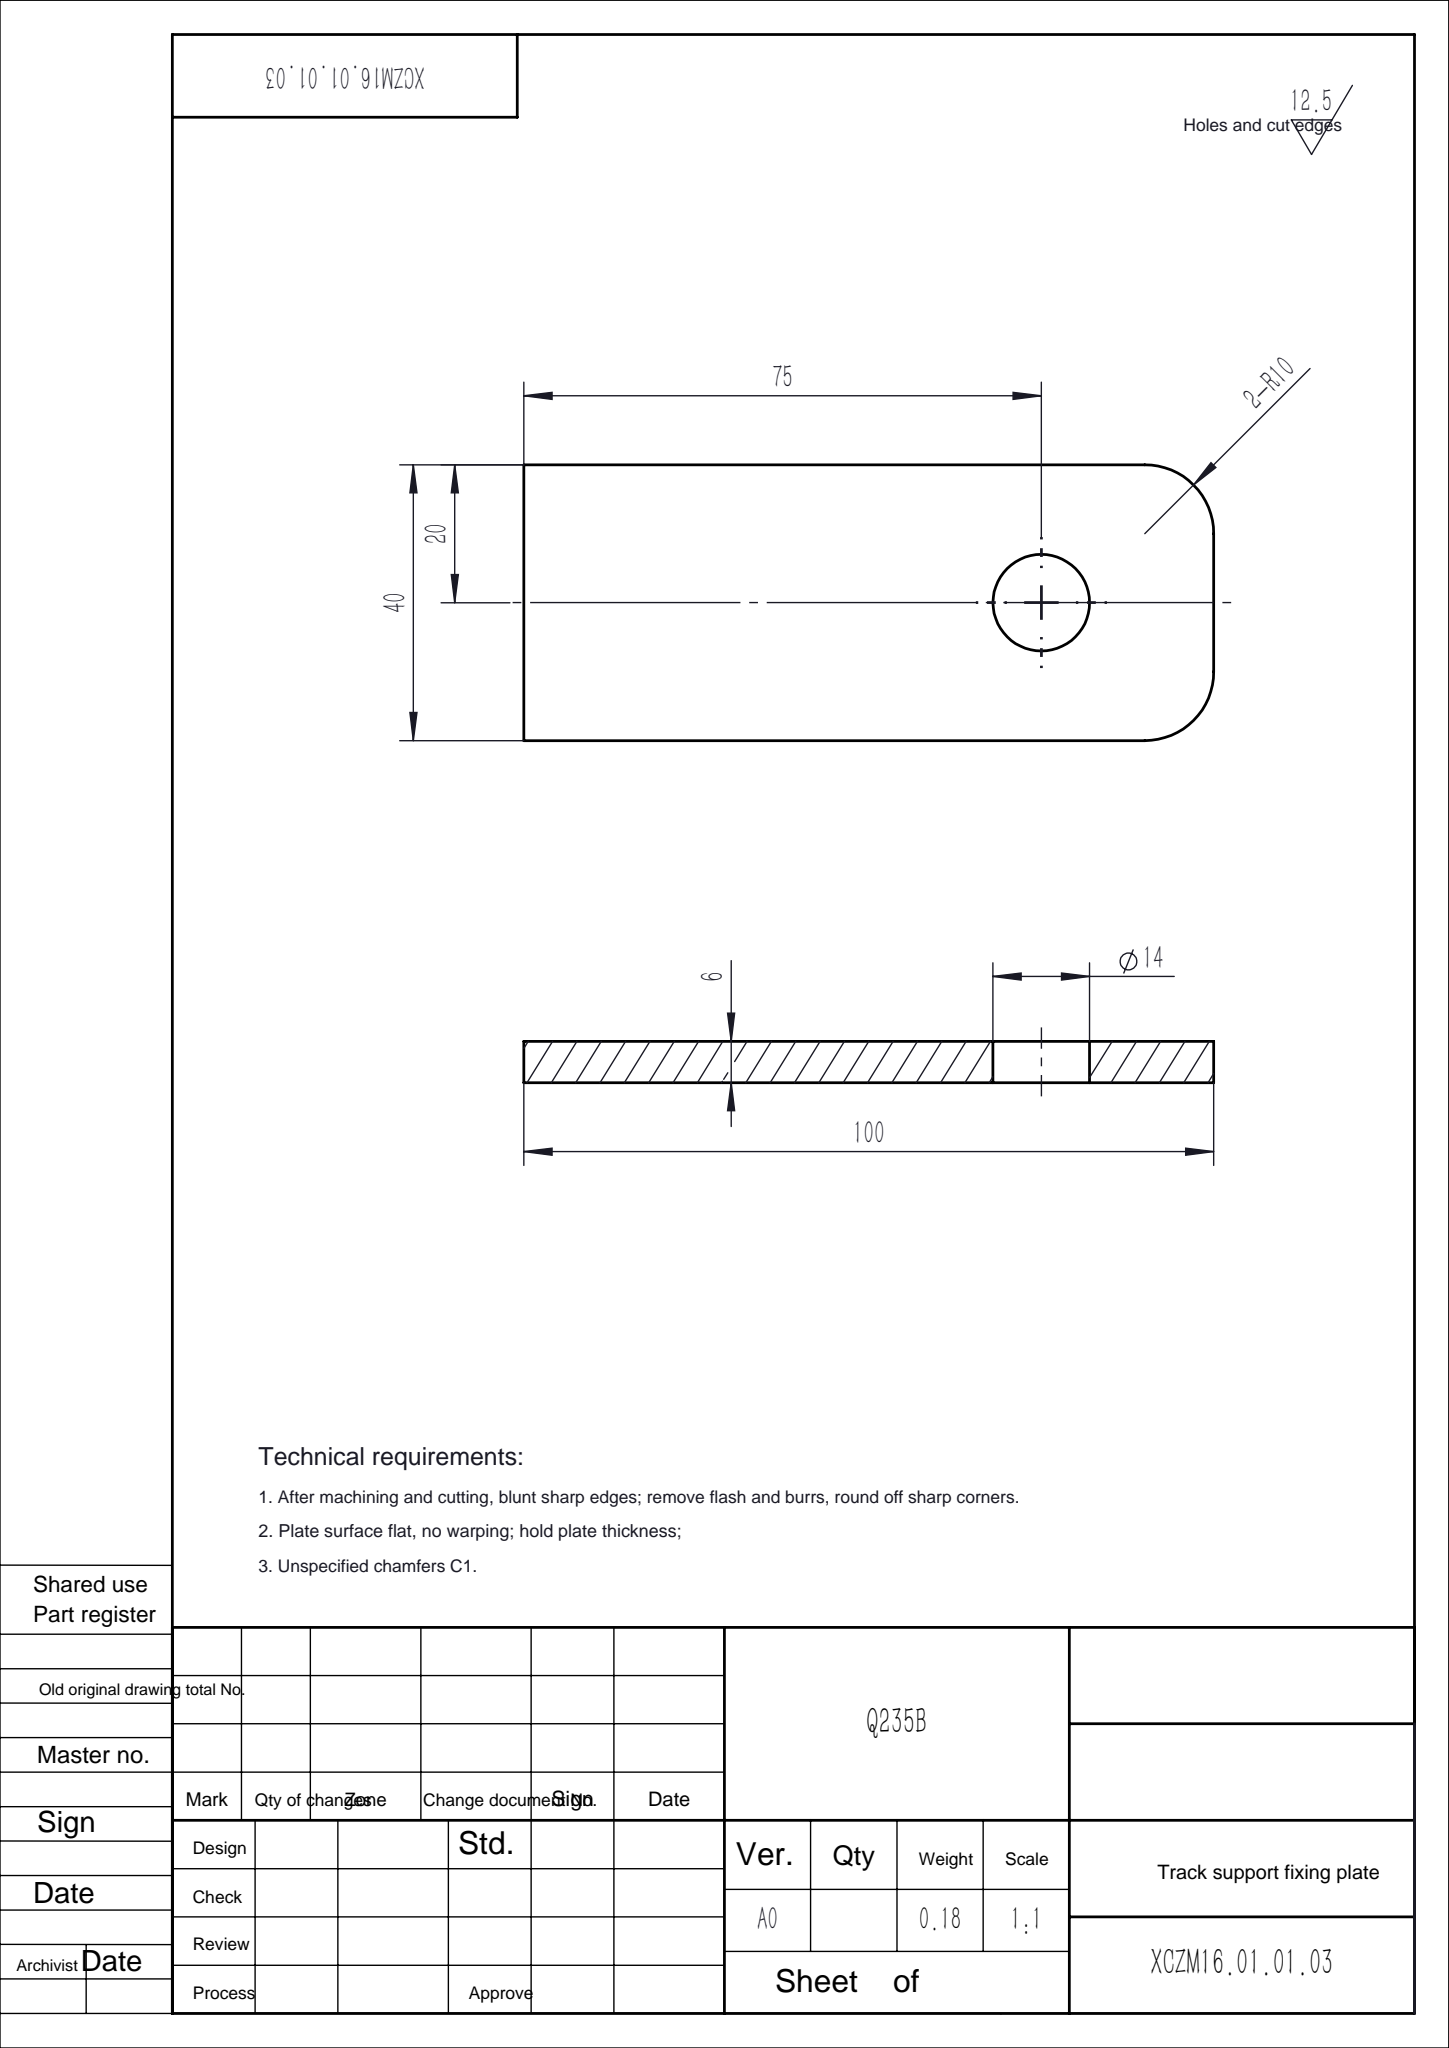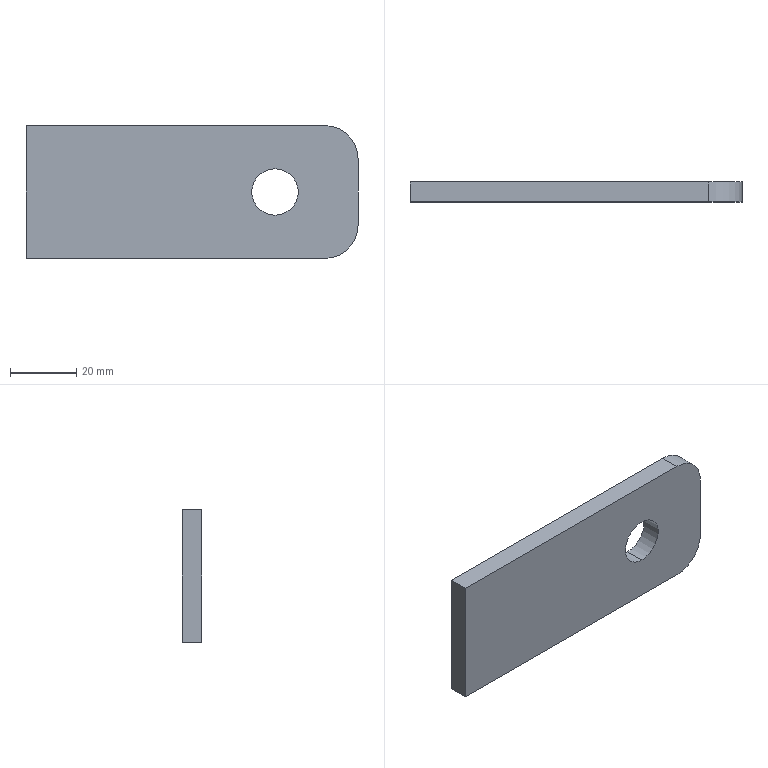Part | SolidWorks | features Extrusion 1 | 1 solid | 10 faces | box 100 x 6 x 40 mm | volume 22819 mm3 | plane 6 | cylinder 4 | commonest cylinder face diameters 14 x2 20 x2
STEP:
#1=CARTESIAN_POINT('',(25.,6.,-7.));
#2=VERTEX_POINT('',#1);
#3=CARTESIAN_POINT('',(25.,6.,7.));
#4=VERTEX_POINT('',#3);
#5=CARTESIAN_POINT('',(25.,6.,0.));
#6=DIRECTION('',(0.,1.,0.));
#7=DIRECTION('',(0.,0.,1.));
#8=AXIS2_PLACEMENT_3D('',#5,#6,#7);
#9=CIRCLE('',#8,7.);
#10=EDGE_CURVE('',#2,#4,#9,.T.);
#11=ORIENTED_EDGE('',*,*,#10,.T.);
#12=CARTESIAN_POINT('',(25.,0.,7.));
#13=VERTEX_POINT('',#12);
#14=CARTESIAN_POINT('',(25.,6.,7.));
#15=DIRECTION('',(0.,-1.,0.));
#16=VECTOR('',#15,1000.);
#17=LINE('',#14,#16);
#18=EDGE_CURVE('',#4,#13,#17,.T.);
#19=ORIENTED_EDGE('',*,*,#18,.T.);
#20=CARTESIAN_POINT('',(25.,0.,-7.));
#21=VERTEX_POINT('',#20);
#22=CARTESIAN_POINT('',(25.,0.,0.));
#23=DIRECTION('',(0.,1.,0.));
#24=DIRECTION('',(0.,0.,1.));
#25=AXIS2_PLACEMENT_3D('',#22,#23,#24);
#26=CIRCLE('',#25,7.);
#27=EDGE_CURVE('',#21,#13,#26,.T.);
#28=ORIENTED_EDGE('',*,*,#27,.F.);
#29=CARTESIAN_POINT('',(25.,6.,-7.));
#30=DIRECTION('',(0.,-1.,0.));
#31=VECTOR('',#30,1000.);
#32=LINE('',#29,#31);
#33=EDGE_CURVE('',#2,#21,#32,.T.);
#34=ORIENTED_EDGE('',*,*,#33,.F.);
#35=EDGE_LOOP('',(#11,#19,#28,#34));
#36=FACE_OUTER_BOUND('',#35,.T.);
#37=CARTESIAN_POINT('',(25.,6.,0.));
#38=DIRECTION('',(0.,-1.,0.));
#39=DIRECTION('',(0.,0.,-1.));
#40=AXIS2_PLACEMENT_3D('',#37,#38,#39);
#41=CYLINDRICAL_SURFACE('',#40,7.);
#42=ADVANCED_FACE('',(#36),#41,.F.);
#43=CARTESIAN_POINT('',(-50.,6.,-20.));
#44=VERTEX_POINT('',#43);
#45=CARTESIAN_POINT('',(-50.,6.,20.));
#46=VERTEX_POINT('',#45);
#47=CARTESIAN_POINT('',(-50.,6.,20.));
#48=DIRECTION('',(0.,0.,1.));
#49=VECTOR('',#48,1000.);
#50=LINE('',#47,#49);
#51=EDGE_CURVE('',#44,#46,#50,.T.);
#52=ORIENTED_EDGE('',*,*,#51,.T.);
#53=CARTESIAN_POINT('',(40.,6.,20.));
#54=VERTEX_POINT('',#53);
#55=CARTESIAN_POINT('',(40.,6.,20.));
#56=DIRECTION('',(1.,0.,0.));
#57=VECTOR('',#56,1000.);
#58=LINE('',#55,#57);
#59=EDGE_CURVE('',#46,#54,#58,.T.);
#60=ORIENTED_EDGE('',*,*,#59,.T.);
#61=CARTESIAN_POINT('',(50.,6.,10.));
#62=VERTEX_POINT('',#61);
#63=CARTESIAN_POINT('',(40.,6.,10.));
#64=DIRECTION('',(0.,1.,0.));
#65=DIRECTION('',(0.,0.,1.));
#66=AXIS2_PLACEMENT_3D('',#63,#64,#65);
#67=CIRCLE('',#66,10.);
#68=EDGE_CURVE('',#54,#62,#67,.T.);
#69=ORIENTED_EDGE('',*,*,#68,.T.);
#70=CARTESIAN_POINT('',(50.,6.,-10.));
#71=VERTEX_POINT('',#70);
#72=CARTESIAN_POINT('',(50.,6.,10.));
#73=DIRECTION('',(0.,0.,-1.));
#74=VECTOR('',#73,1000.);
#75=LINE('',#72,#74);
#76=EDGE_CURVE('',#62,#71,#75,.T.);
#77=ORIENTED_EDGE('',*,*,#76,.T.);
#78=CARTESIAN_POINT('',(40.,6.,-20.));
#79=VERTEX_POINT('',#78);
#80=CARTESIAN_POINT('',(40.,6.,-10.));
#81=DIRECTION('',(0.,1.,0.));
#82=DIRECTION('',(0.,0.,1.));
#83=AXIS2_PLACEMENT_3D('',#80,#81,#82);
#84=CIRCLE('',#83,10.);
#85=EDGE_CURVE('',#71,#79,#84,.T.);
#86=ORIENTED_EDGE('',*,*,#85,.T.);
#87=CARTESIAN_POINT('',(40.,6.,-20.));
#88=DIRECTION('',(-1.,0.,0.));
#89=VECTOR('',#88,1000.);
#90=LINE('',#87,#89);
#91=EDGE_CURVE('',#79,#44,#90,.T.);
#92=ORIENTED_EDGE('',*,*,#91,.T.);
#93=EDGE_LOOP('',(#52,#60,#69,#77,#86,#92));
#94=FACE_OUTER_BOUND('',#93,.T.);
#95=ORIENTED_EDGE('',*,*,#10,.F.);
#96=CARTESIAN_POINT('',(25.,6.,0.));
#97=DIRECTION('',(0.,1.,0.));
#98=DIRECTION('',(0.,0.,1.));
#99=AXIS2_PLACEMENT_3D('',#96,#97,#98);
#100=CIRCLE('',#99,7.);
#101=EDGE_CURVE('',#4,#2,#100,.T.);
#102=ORIENTED_EDGE('',*,*,#101,.F.);
#103=EDGE_LOOP('',(#95,#102));
#104=FACE_BOUND('',#103,.T.);
#105=CARTESIAN_POINT('',(40.,6.,-10.));
#106=DIRECTION('',(0.,1.,0.));
#107=DIRECTION('',(0.,0.,1.));
#108=AXIS2_PLACEMENT_3D('',#105,#106,#107);
#109=PLANE('',#108);
#110=ADVANCED_FACE('',(#94,#104),#109,.T.);
#111=CARTESIAN_POINT('',(-50.,0.,-20.));
#112=VERTEX_POINT('',#111);
#113=CARTESIAN_POINT('',(-50.,0.,20.));
#114=VERTEX_POINT('',#113);
#115=CARTESIAN_POINT('',(-50.,0.,20.));
#116=DIRECTION('',(0.,0.,1.));
#117=VECTOR('',#116,1000.);
#118=LINE('',#115,#117);
#119=EDGE_CURVE('',#112,#114,#118,.T.);
#120=ORIENTED_EDGE('',*,*,#119,.F.);
#121=CARTESIAN_POINT('',(40.,0.,-20.));
#122=VERTEX_POINT('',#121);
#123=CARTESIAN_POINT('',(40.,0.,-20.));
#124=DIRECTION('',(-1.,0.,0.));
#125=VECTOR('',#124,1000.);
#126=LINE('',#123,#125);
#127=EDGE_CURVE('',#122,#112,#126,.T.);
#128=ORIENTED_EDGE('',*,*,#127,.F.);
#129=CARTESIAN_POINT('',(50.,0.,-10.));
#130=VERTEX_POINT('',#129);
#131=CARTESIAN_POINT('',(40.,0.,-10.));
#132=DIRECTION('',(0.,1.,0.));
#133=DIRECTION('',(0.,0.,1.));
#134=AXIS2_PLACEMENT_3D('',#131,#132,#133);
#135=CIRCLE('',#134,10.);
#136=EDGE_CURVE('',#130,#122,#135,.T.);
#137=ORIENTED_EDGE('',*,*,#136,.F.);
#138=CARTESIAN_POINT('',(50.,0.,10.));
#139=VERTEX_POINT('',#138);
#140=CARTESIAN_POINT('',(50.,0.,10.));
#141=DIRECTION('',(0.,0.,-1.));
#142=VECTOR('',#141,1000.);
#143=LINE('',#140,#142);
#144=EDGE_CURVE('',#139,#130,#143,.T.);
#145=ORIENTED_EDGE('',*,*,#144,.F.);
#146=CARTESIAN_POINT('',(40.,0.,20.));
#147=VERTEX_POINT('',#146);
#148=CARTESIAN_POINT('',(40.,0.,10.));
#149=DIRECTION('',(0.,1.,0.));
#150=DIRECTION('',(0.,0.,1.));
#151=AXIS2_PLACEMENT_3D('',#148,#149,#150);
#152=CIRCLE('',#151,10.);
#153=EDGE_CURVE('',#147,#139,#152,.T.);
#154=ORIENTED_EDGE('',*,*,#153,.F.);
#155=CARTESIAN_POINT('',(40.,0.,20.));
#156=DIRECTION('',(1.,0.,0.));
#157=VECTOR('',#156,1000.);
#158=LINE('',#155,#157);
#159=EDGE_CURVE('',#114,#147,#158,.T.);
#160=ORIENTED_EDGE('',*,*,#159,.F.);
#161=EDGE_LOOP('',(#120,#128,#137,#145,#154,#160));
#162=FACE_OUTER_BOUND('',#161,.T.);
#163=ORIENTED_EDGE('',*,*,#27,.T.);
#164=CARTESIAN_POINT('',(25.,0.,0.));
#165=DIRECTION('',(0.,1.,0.));
#166=DIRECTION('',(0.,0.,1.));
#167=AXIS2_PLACEMENT_3D('',#164,#165,#166);
#168=CIRCLE('',#167,7.);
#169=EDGE_CURVE('',#13,#21,#168,.T.);
#170=ORIENTED_EDGE('',*,*,#169,.T.);
#171=EDGE_LOOP('',(#163,#170));
#172=FACE_BOUND('',#171,.T.);
#173=CARTESIAN_POINT('',(40.,0.,-10.));
#174=DIRECTION('',(0.,1.,0.));
#175=DIRECTION('',(0.,0.,1.));
#176=AXIS2_PLACEMENT_3D('',#173,#174,#175);
#177=PLANE('',#176);
#178=ADVANCED_FACE('',(#162,#172),#177,.F.);
#179=ORIENTED_EDGE('',*,*,#119,.T.);
#180=CARTESIAN_POINT('',(-50.,6.,20.));
#181=DIRECTION('',(0.,-1.,0.));
#182=VECTOR('',#181,1000.);
#183=LINE('',#180,#182);
#184=EDGE_CURVE('',#46,#114,#183,.T.);
#185=ORIENTED_EDGE('',*,*,#184,.F.);
#186=ORIENTED_EDGE('',*,*,#51,.F.);
#187=CARTESIAN_POINT('',(-50.,6.,-20.));
#188=DIRECTION('',(0.,-1.,0.));
#189=VECTOR('',#188,1000.);
#190=LINE('',#187,#189);
#191=EDGE_CURVE('',#44,#112,#190,.T.);
#192=ORIENTED_EDGE('',*,*,#191,.T.);
#193=EDGE_LOOP('',(#179,#185,#186,#192));
#194=FACE_OUTER_BOUND('',#193,.T.);
#195=CARTESIAN_POINT('',(-50.,6.,20.));
#196=DIRECTION('',(1.,0.,0.));
#197=DIRECTION('',(0.,0.,-1.));
#198=AXIS2_PLACEMENT_3D('',#195,#196,#197);
#199=PLANE('',#198);
#200=ADVANCED_FACE('',(#194),#199,.F.);
#201=ORIENTED_EDGE('',*,*,#159,.T.);
#202=CARTESIAN_POINT('',(40.,6.,20.));
#203=DIRECTION('',(0.,-1.,0.));
#204=VECTOR('',#203,1000.);
#205=LINE('',#202,#204);
#206=EDGE_CURVE('',#54,#147,#205,.T.);
#207=ORIENTED_EDGE('',*,*,#206,.F.);
#208=ORIENTED_EDGE('',*,*,#59,.F.);
#209=ORIENTED_EDGE('',*,*,#184,.T.);
#210=EDGE_LOOP('',(#201,#207,#208,#209));
#211=FACE_OUTER_BOUND('',#210,.T.);
#212=CARTESIAN_POINT('',(40.,6.,20.));
#213=DIRECTION('',(0.,0.,-1.));
#214=DIRECTION('',(-1.,0.,0.));
#215=AXIS2_PLACEMENT_3D('',#212,#213,#214);
#216=PLANE('',#215);
#217=ADVANCED_FACE('',(#211),#216,.F.);
#218=ORIENTED_EDGE('',*,*,#153,.T.);
#219=CARTESIAN_POINT('',(50.,6.,10.));
#220=DIRECTION('',(0.,-1.,0.));
#221=VECTOR('',#220,1000.);
#222=LINE('',#219,#221);
#223=EDGE_CURVE('',#62,#139,#222,.T.);
#224=ORIENTED_EDGE('',*,*,#223,.F.);
#225=ORIENTED_EDGE('',*,*,#68,.F.);
#226=ORIENTED_EDGE('',*,*,#206,.T.);
#227=EDGE_LOOP('',(#218,#224,#225,#226));
#228=FACE_OUTER_BOUND('',#227,.T.);
#229=CARTESIAN_POINT('',(40.,6.,10.));
#230=DIRECTION('',(0.,-1.,0.));
#231=DIRECTION('',(0.,0.,-1.));
#232=AXIS2_PLACEMENT_3D('',#229,#230,#231);
#233=CYLINDRICAL_SURFACE('',#232,10.);
#234=ADVANCED_FACE('',(#228),#233,.T.);
#235=ORIENTED_EDGE('',*,*,#144,.T.);
#236=CARTESIAN_POINT('',(50.,6.,-10.));
#237=DIRECTION('',(0.,-1.,0.));
#238=VECTOR('',#237,1000.);
#239=LINE('',#236,#238);
#240=EDGE_CURVE('',#71,#130,#239,.T.);
#241=ORIENTED_EDGE('',*,*,#240,.F.);
#242=ORIENTED_EDGE('',*,*,#76,.F.);
#243=ORIENTED_EDGE('',*,*,#223,.T.);
#244=EDGE_LOOP('',(#235,#241,#242,#243));
#245=FACE_OUTER_BOUND('',#244,.T.);
#246=CARTESIAN_POINT('',(50.,6.,10.));
#247=DIRECTION('',(-1.,0.,0.));
#248=DIRECTION('',(0.,0.,1.));
#249=AXIS2_PLACEMENT_3D('',#246,#247,#248);
#250=PLANE('',#249);
#251=ADVANCED_FACE('',(#245),#250,.F.);
#252=ORIENTED_EDGE('',*,*,#136,.T.);
#253=CARTESIAN_POINT('',(40.,6.,-20.));
#254=DIRECTION('',(0.,-1.,0.));
#255=VECTOR('',#254,1000.);
#256=LINE('',#253,#255);
#257=EDGE_CURVE('',#79,#122,#256,.T.);
#258=ORIENTED_EDGE('',*,*,#257,.F.);
#259=ORIENTED_EDGE('',*,*,#85,.F.);
#260=ORIENTED_EDGE('',*,*,#240,.T.);
#261=EDGE_LOOP('',(#252,#258,#259,#260));
#262=FACE_OUTER_BOUND('',#261,.T.);
#263=CARTESIAN_POINT('',(40.,6.,-10.));
#264=DIRECTION('',(0.,-1.,0.));
#265=DIRECTION('',(0.,0.,-1.));
#266=AXIS2_PLACEMENT_3D('',#263,#264,#265);
#267=CYLINDRICAL_SURFACE('',#266,10.);
#268=ADVANCED_FACE('',(#262),#267,.T.);
#269=ORIENTED_EDGE('',*,*,#127,.T.);
#270=ORIENTED_EDGE('',*,*,#191,.F.);
#271=ORIENTED_EDGE('',*,*,#91,.F.);
#272=ORIENTED_EDGE('',*,*,#257,.T.);
#273=EDGE_LOOP('',(#269,#270,#271,#272));
#274=FACE_OUTER_BOUND('',#273,.T.);
#275=CARTESIAN_POINT('',(40.,6.,-20.));
#276=DIRECTION('',(0.,0.,1.));
#277=DIRECTION('',(1.,0.,0.));
#278=AXIS2_PLACEMENT_3D('',#275,#276,#277);
#279=PLANE('',#278);
#280=ADVANCED_FACE('',(#274),#279,.F.);
#281=ORIENTED_EDGE('',*,*,#18,.F.);
#282=ORIENTED_EDGE('',*,*,#101,.T.);
#283=ORIENTED_EDGE('',*,*,#33,.T.);
#284=ORIENTED_EDGE('',*,*,#169,.F.);
#285=EDGE_LOOP('',(#281,#282,#283,#284));
#286=FACE_OUTER_BOUND('',#285,.T.);
#287=CARTESIAN_POINT('',(25.,6.,0.));
#288=DIRECTION('',(0.,-1.,0.));
#289=DIRECTION('',(0.,0.,-1.));
#290=AXIS2_PLACEMENT_3D('',#287,#288,#289);
#291=CYLINDRICAL_SURFACE('',#290,7.);
#292=ADVANCED_FACE('',(#286),#291,.F.);
#293=CLOSED_SHELL('',(#42,#110,#178,#200,#217,#234,#251,#268,#280,#292));
#294=MANIFOLD_SOLID_BREP('',#293);
#295=CARTESIAN_POINT('',(0.,0.,0.));
#296=DIRECTION('',(0.,0.,1.));
#297=DIRECTION('',(1.,0.,0.));
#298=AXIS2_PLACEMENT_3D('',#295,#296,#297);
#299=(LENGTH_UNIT()NAMED_UNIT(*)SI_UNIT(.MILLI.,.METRE.));
#300=UNCERTAINTY_MEASURE_WITH_UNIT(LENGTH_MEASURE(0.00001),#299,'','');
#301=(NAMED_UNIT(*)PLANE_ANGLE_UNIT()SI_UNIT($,.RADIAN.));
#302=(NAMED_UNIT(*)SI_UNIT($,.STERADIAN.)SOLID_ANGLE_UNIT());
#303=(GEOMETRIC_REPRESENTATION_CONTEXT(3)GLOBAL_UNCERTAINTY_ASSIGNED_CONTEXT((#300))GLOBAL_UNIT_ASSIGNED_CONTEXT((#299,#301,#302))REPRESENTATION_CONTEXT('',''));
#304=ADVANCED_BREP_SHAPE_REPRESENTATION('',(#294,#298),#303);